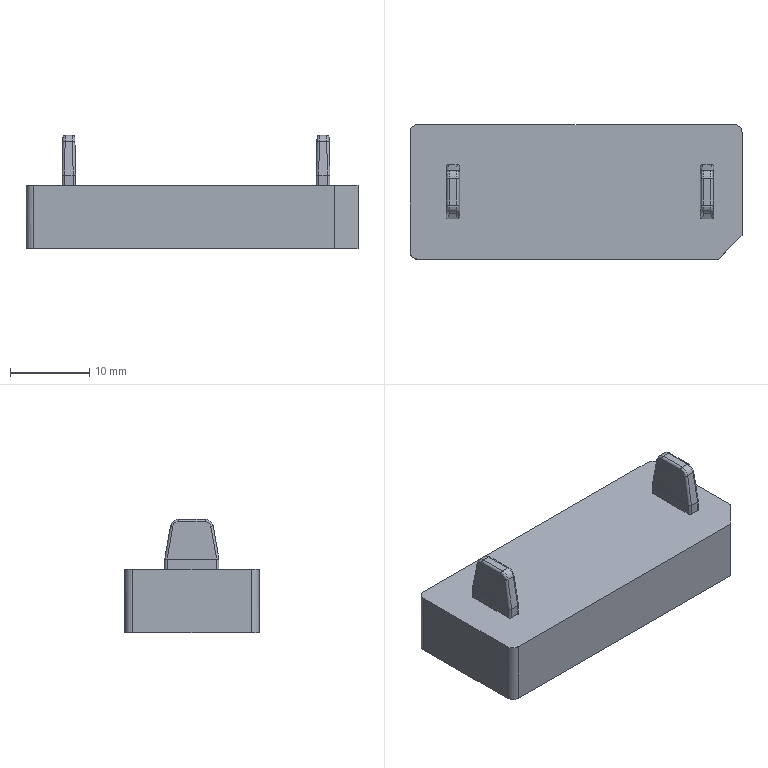NC program | PowerMill | posted by the shop | part box 42 x 17 x 14.346 mm
Lines 4335 to 5367 of 86217:
( TOOL ID   R1_1_1 )
( TOOL DIA. 2. TIP RAD 1. LENGTH 57.2 )
( Z = -2.198 )
T4 M6
T5
G91 G28 Z0
G0 G90 G54
M08
S18000 M3
X0 Y0 M8
G43 Z10.796 H4
X18.04 Y-3.123
Z-.918
G1 Z-2.118 F1200
X18.031 Y-3.133 Z-2.099 F2000
X18.016 Y-3.147 Z-2.074
X17.999 Y-3.164 Z-2.052
X17.932 Y-3.231 Z-2.005
X17.868 Y-3.296 Z-2.017
X17.813 Y-3.351 Z-2.056
X17.796 Y-3.368 Z-2.078
X17.67 Y-3.451 Z-2.068
X17.685 Y-3.436 Z-2.032
X17.706 Y-3.415 Z-1.992
X17.735 Y-3.386 Z-1.94
X17.754 Y-3.367 Z-1.908
X17.773 Y-3.348 Z-1.882
X17.792 Y-3.329 Z-1.86
X17.814 Y-3.307 Z-1.841
X17.837 Y-3.284 Z-1.825
X17.841 Y-3.28 Z-1.823
X17.905 Y-3.216 Z-1.806
X17.973 Y-3.148 Z-1.83
X18.035 Y-3.086 Z-1.898
X18.048 Y-3.073 Z-1.921
X18.061 Y-3.06 Z-1.949
X18.075 Y-3.045 Z-1.985
X18.092 Y-3.029 Z-2.033
X18.104 Y-3.016 Z-2.074
X18.113 Y-3.008 Z-2.106
X18.12 Y-3.001 Z-2.134
X18.122 Y-2.999 Z-2.142
X18.168 Y-2.91 Z-2.158
X18.165 Y-2.914 Z-2.137
X18.154 Y-2.924 Z-2.078
X18.143 Y-2.935 Z-2.023
X18.132 Y-2.947 Z-1.973
X18.12 Y-2.959 Z-1.928
X18.107 Y-2.972 Z-1.888
X18.093 Y-2.985 Z-1.851
X18.078 Y-3. Z-1.819
X18.062 Y-3.017 Z-1.79
X18.004 Y-3.075 Z-1.719
X17.937 Y-3.142 Z-1.681
X17.869 Y-3.21 Z-1.674
X17.858 Y-3.22 Z-1.677
X17.832 Y-3.246 Z-1.684
X17.807 Y-3.271 Z-1.695
X17.783 Y-3.296 Z-1.709
X17.76 Y-3.319 Z-1.726
X17.738 Y-3.341 Z-1.747
X17.716 Y-3.362 Z-1.771
X17.696 Y-3.383 Z-1.8
X17.675 Y-3.403 Z-1.834
X17.655 Y-3.423 Z-1.873
X17.634 Y-3.444 Z-1.921
X17.611 Y-3.468 Z-1.979
X17.581 Y-3.497 Z-2.059
X17.507 Y-3.529 Z-2.053
X17.52 Y-3.516 Z-2.012
X17.537 Y-3.499 Z-1.959
X17.559 Y-3.477 Z-1.893
X17.577 Y-3.459 Z-1.844
X17.594 Y-3.442 Z-1.805
X17.609 Y-3.427 Z-1.773
X17.623 Y-3.413 Z-1.75
X17.639 Y-3.397 Z-1.725
X17.661 Y-3.375 Z-1.696
X17.687 Y-3.349 Z-1.664
X17.712 Y-3.324 Z-1.638
X17.735 Y-3.301 Z-1.619
X17.756 Y-3.28 Z-1.605
X17.776 Y-3.26 Z-1.594
X17.796 Y-3.24 Z-1.585
X17.817 Y-3.219 Z-1.578
X17.84 Y-3.196 Z-1.571
X17.861 Y-3.175 Z-1.569
X17.882 Y-3.154
X17.902 Y-3.134 Z-1.57
X17.921 Y-3.115 Z-1.574
X17.944 Y-3.092 Z-1.583
X17.97 Y-3.066 Z-1.594
X18.034 Y-3.002 Z-1.644
X18.089 Y-2.947 Z-1.721
X18.106 Y-2.93 Z-1.756
X18.122 Y-2.914 Z-1.792
X18.136 Y-2.9 Z-1.83
X18.149 Y-2.887 Z-1.872
X18.16 Y-2.876 Z-1.918
X18.171 Y-2.865 Z-1.973
X18.18 Y-2.856 Z-2.031
X18.188 Y-2.848 Z-2.086
X18.195 Y-2.841 Z-2.138
X18.2 Y-2.836 Z-2.171
X18.223 Y-2.771 Z-2.183
X18.219 Y-2.775 Z-2.14
X18.212 Y-2.782 Z-2.072
X18.204 Y-2.79 Z-2.008
X18.196 Y-2.798 Z-1.949
X18.186 Y-2.807 Z-1.897
X18.175 Y-2.818 Z-1.846
X18.164 Y-2.83 Z-1.803
X18.149 Y-2.844 Z-1.756
X18.133 Y-2.86 Z-1.713
X18.116 Y-2.878 Z-1.675
X18.097 Y-2.896 Z-1.641
X18.077 Y-2.917 Z-1.609
X18.056 Y-2.937 Z-1.581
X18.033 Y-2.961 Z-1.556
X18.008 Y-2.986 Z-1.534
X17.982 Y-3.012 Z-1.515
X17.955 Y-3.038 Z-1.501
X17.928 Y-3.066 Z-1.49
X17.9 Y-3.093 Z-1.483
X17.872 Y-3.121 Z-1.48
X17.842 Y-3.151 Z-1.481
X17.813 Y-3.181 Z-1.486
X17.783 Y-3.211 Z-1.494
X17.753 Y-3.241 Z-1.507
X17.723 Y-3.27 Z-1.523
X17.694 Y-3.299 Z-1.544
X17.666 Y-3.328 Z-1.569
X17.638 Y-3.356 Z-1.597
X17.611 Y-3.382 Z-1.63
X17.587 Y-3.406 Z-1.663
X17.566 Y-3.428 Z-1.698
X17.545 Y-3.448 Z-1.736
X17.527 Y-3.467 Z-1.777
X17.509 Y-3.485 Z-1.822
X17.492 Y-3.502 Z-1.871
X17.475 Y-3.519 Z-1.926
X17.457 Y-3.536 Z-1.99
X17.441 Y-3.553 Z-2.047
X17.381 Y-3.57 Z-2.043
X17.399 Y-3.552 Z-1.974
X17.416 Y-3.535 Z-1.905
X17.431 Y-3.52 Z-1.851
X17.446 Y-3.505 Z-1.805
X17.462 Y-3.489 Z-1.762
X17.479 Y-3.472 Z-1.722
X17.497 Y-3.454 Z-1.684
X17.517 Y-3.434 Z-1.647
X17.539 Y-3.412 Z-1.611
X17.565 Y-3.386 Z-1.573
X17.593 Y-3.358 Z-1.539
X17.623 Y-3.328 Z-1.508
X17.653 Y-3.298 Z-1.481
X17.684 Y-3.267 Z-1.458
X17.716 Y-3.236 Z-1.439
X17.747 Y-3.204 Z-1.424
X17.779 Y-3.172 Z-1.413
X17.811 Y-3.141 Z-1.406
X17.842 Y-3.109 Z-1.403
X17.873 Y-3.078 Z-1.404
X17.903 Y-3.048 Z-1.408
X17.933 Y-3.018 Z-1.417
X17.961 Y-2.99 Z-1.429
X17.989 Y-2.962 Z-1.445
X18.016 Y-2.936 Z-1.465
X18.041 Y-2.91 Z-1.488
X18.065 Y-2.886 Z-1.515
X18.087 Y-2.864 Z-1.546
X18.109 Y-2.843 Z-1.58
X18.128 Y-2.823 Z-1.617
X18.146 Y-2.805 Z-1.657
X18.163 Y-2.788 Z-1.701
X18.177 Y-2.774 Z-1.748
X18.19 Y-2.761 Z-1.797
X18.199 Y-2.753 Z-1.836
X18.207 Y-2.744 Z-1.882
X18.215 Y-2.737 Z-1.928
X18.221 Y-2.73 Z-1.976
X18.227 Y-2.725 Z-2.034
X18.231 Y-2.72 Z-2.081
X18.235 Y-2.716 Z-2.129
X18.239 Y-2.712 Z-2.176
X18.241 Y-2.71 Z-2.193
X18.254 Y-2.655
X18.252 Y-2.656 Z-2.176
X18.247 Y-2.662 Z-2.096
X18.24 Y-2.669 Z-2.012
X18.232 Y-2.676 Z-1.934
X18.223 Y-2.685 Z-1.865
X18.213 Y-2.696 Z-1.802
X18.2 Y-2.709 Z-1.743
X18.188 Y-2.721 Z-1.697
X18.172 Y-2.736 Z-1.648
X18.155 Y-2.754 Z-1.602
X18.136 Y-2.773 Z-1.56
X18.115 Y-2.793 Z-1.522
X18.093 Y-2.815 Z-1.487
X18.07 Y-2.839 Z-1.456
X18.045 Y-2.863 Z-1.428
X18.019 Y-2.889 Z-1.404
X17.992 Y-2.917 Z-1.383
X17.964 Y-2.945 Z-1.366
X17.934 Y-2.975 Z-1.352
X17.904 Y-3.005 Z-1.342
X17.873 Y-3.036 Z-1.336
X17.841 Y-3.068 Z-1.333
X17.808 Y-3.1 Z-1.335
X17.775 Y-3.133 Z-1.34
X17.742 Y-3.166 Z-1.349
X17.709 Y-3.2 Z-1.363
X17.676 Y-3.233 Z-1.38
X17.643 Y-3.266 Z-1.402
X17.611 Y-3.298 Z-1.427
X17.58 Y-3.329 Z-1.456
X17.55 Y-3.359 Z-1.489
X17.526 Y-3.383 Z-1.519
X17.5 Y-3.408 Z-1.555
X17.477 Y-3.432 Z-1.592
X17.454 Y-3.454 Z-1.631
X17.434 Y-3.475 Z-1.673
X17.415 Y-3.494 Z-1.717
X17.398 Y-3.511 Z-1.763
X17.382 Y-3.527 Z-1.813
X17.366 Y-3.542 Z-1.866
X17.352 Y-3.557 Z-1.924
X17.338 Y-3.571 Z-1.985
X17.325 Y-3.584 Z-2.039
X17.272 Y-3.594 Z-2.036
X17.286 Y-3.581 Z-1.974
X17.301 Y-3.566 Z-1.907
X17.318 Y-3.549 Z-1.837
X17.334 Y-3.532 Z-1.778
X17.351 Y-3.515 Z-1.728
X17.368 Y-3.498 Z-1.682
X17.387 Y-3.479 Z-1.639
X17.407 Y-3.459 Z-1.599
X17.428 Y-3.438 Z-1.56
X17.452 Y-3.415 Z-1.521
X17.48 Y-3.386 Z-1.48
X17.51 Y-3.356 Z-1.441
X17.542 Y-3.324 Z-1.406
X17.575 Y-3.292 Z-1.375
X17.608 Y-3.258 Z-1.348
X17.642 Y-3.224 Z-1.325
X17.677 Y-3.19 Z-1.306
X17.711 Y-3.155 Z-1.291
X17.745 Y-3.121 Z-1.28
X17.78 Y-3.087 Z-1.273
X17.813 Y-3.053 Z-1.27
X17.847 Y-3.02 Z-1.271
X17.88 Y-2.987 Z-1.276
X17.91 Y-2.956 Z-1.284
X17.941 Y-2.925 Z-1.296
X17.972 Y-2.895 Z-1.311
X18. Y-2.866 Z-1.33
X18.028 Y-2.838 Z-1.352
X18.054 Y-2.812 Z-1.378
X18.079 Y-2.787 Z-1.407
X18.103 Y-2.763 Z-1.44
X18.125 Y-2.741 Z-1.476
X18.146 Y-2.721 Z-1.515
X18.164 Y-2.702 Z-1.559
X18.182 Y-2.685 Z-1.605
X18.197 Y-2.669 Z-1.655
X18.211 Y-2.656 Z-1.709
X18.222 Y-2.644 Z-1.764
X18.231 Y-2.635 Z-1.816
X18.239 Y-2.628 Z-1.87
X18.245 Y-2.621 Z-1.923
X18.25 Y-2.616 Z-1.985
X18.254 Y-2.612 Z-2.039
X18.257 Y-2.609 Z-2.093
X18.26 Y-2.606 Z-2.148
X18.262 Y-2.605 Z-2.173
X18.268 Y-2.556 Z-2.147
X18.267 Y-2.557 Z-2.131
X18.262 Y-2.562 Z-2.033
X18.256 Y-2.567 Z-1.94
X18.25 Y-2.574 Z-1.865
X18.241 Y-2.583 Z-1.798
X18.231 Y-2.593 Z-1.733
X18.219 Y-2.605 Z-1.675
X18.206 Y-2.618 Z-1.62
X18.19 Y-2.634 Z-1.568
X18.173 Y-2.651 Z-1.52
X18.154 Y-2.67 Z-1.475
X18.134 Y-2.69 Z-1.436
X18.112 Y-2.712 Z-1.399
X18.088 Y-2.736 Z-1.365
X18.062 Y-2.761 Z-1.334
X18.035 Y-2.789 Z-1.306
X18.007 Y-2.817 Z-1.282
X17.977 Y-2.847 Z-1.261
X17.946 Y-2.878 Z-1.244
X17.914 Y-2.91 Z-1.23
X17.881 Y-2.943 Z-1.22
X17.848 Y-2.976 Z-1.214
X17.814 Y-3.01 Z-1.212
X17.779 Y-3.044 Z-1.213
X17.745 Y-3.079 Z-1.218
X17.709 Y-3.115 Z-1.228
X17.673 Y-3.151 Z-1.241
X17.638 Y-3.186 Z-1.258
X17.602 Y-3.222 Z-1.279
X17.567 Y-3.256 Z-1.305
X17.533 Y-3.291 Z-1.334
X17.499 Y-3.325 Z-1.368
X17.468 Y-3.356 Z-1.403
X17.438 Y-3.386 Z-1.442
X17.409 Y-3.415 Z-1.484
X17.382 Y-3.442 Z-1.531
X17.355 Y-3.469 Z-1.581
X17.335 Y-3.489 Z-1.625
X17.317 Y-3.507 Z-1.668
X17.301 Y-3.523 Z-1.712
X17.286 Y-3.538 Z-1.756
X17.273 Y-3.551 Z-1.802
X17.262 Y-3.562 Z-1.848
X17.251 Y-3.573 Z-1.896
X17.241 Y-3.583 Z-1.944
X17.231 Y-3.593 Z-1.992
X17.222 Y-3.602 Z-2.034
X17.174 Y-3.608 Z-2.033
X17.195 Y-3.586 Z-1.923
X17.212 Y-3.569 Z-1.845
X17.228 Y-3.553 Z-1.78
X17.245 Y-3.536 Z-1.722
X17.263 Y-3.519 Z-1.67
X17.282 Y-3.5 Z-1.62
X17.302 Y-3.479 Z-1.574
X17.324 Y-3.457 Z-1.529
X17.348 Y-3.433 Z-1.485
X17.374 Y-3.408 Z-1.443
X17.403 Y-3.378 Z-1.399
X17.435 Y-3.347 Z-1.358
X17.468 Y-3.313 Z-1.321
X17.503 Y-3.279 Z-1.287
X17.538 Y-3.243 Z-1.257
X17.575 Y-3.207 Z-1.23
X17.611 Y-3.17 Z-1.208
X17.648 Y-3.133 Z-1.19
X17.685 Y-3.096 Z-1.176
X17.722 Y-3.059 Z-1.166
X17.759 Y-3.023 Z-1.16
X17.795 Y-2.986 Z-1.158
X17.831 Y-2.951 Z-1.16
X17.866 Y-2.916 Z-1.166
X17.9 Y-2.882 Z-1.175
X17.933 Y-2.848 Z-1.188
X17.965 Y-2.816 Z-1.205
X17.996 Y-2.786 Z-1.225
X18.025 Y-2.756 Z-1.248
X18.054 Y-2.728 Z-1.276
X18.08 Y-2.701 Z-1.306
X18.105 Y-2.676 Z-1.34
X18.129 Y-2.652 Z-1.378
X18.151 Y-2.631 Z-1.418
X18.171 Y-2.611 Z-1.462
X18.189 Y-2.592 Z-1.508
X18.205 Y-2.576 Z-1.558
X18.219 Y-2.562 Z-1.61
X18.231 Y-2.55 Z-1.665
X18.241 Y-2.54 Z-1.725
X18.251 Y-2.531 Z-1.792
X18.259 Y-2.523 Z-1.871
X18.265 Y-2.516 Z-1.962
X18.269 Y-2.512 Z-2.045
X18.272 Y-2.509 Z-2.114
X18.273 Z-2.122
X18.275 Y-2.464 Z-2.099
Z-2.085
X18.272 Y-2.467 Z-1.99
X18.266 Y-2.473 Z-1.891
X18.26 Y-2.479 Z-1.808
X18.252 Y-2.487 Z-1.736
X18.243 Y-2.496 Z-1.672
X18.233 Y-2.506 Z-1.615
X18.22 Y-2.519 Z-1.562
X18.206 Y-2.533 Z-1.511
X18.19 Y-2.549 Z-1.462
X18.172 Y-2.567 Z-1.417
X18.152 Y-2.587 Z-1.374
X18.13 Y-2.609 Z-1.334
X18.107 Y-2.632 Z-1.297
X18.082 Y-2.658 Z-1.263
X18.055 Y-2.684 Z-1.232
X18.026 Y-2.713 Z-1.204
X17.996 Y-2.743 Z-1.18
X17.964 Y-2.775 Z-1.159
X17.931 Y-2.808 Z-1.142
X17.897 Y-2.842 Z-1.128
X17.861 Y-2.878 Z-1.117
X17.825 Y-2.914 Z-1.111
X17.788 Y-2.951 Z-1.108
X17.751 Y-2.988 Z-1.109
X17.714 Y-3.025 Z-1.114
X17.676 Y-3.063 Z-1.124
X17.638 Y-3.101 Z-1.137
X17.6 Y-3.139 Z-1.154
X17.562 Y-3.177 Z-1.176
X17.525 Y-3.215 Z-1.201
X17.488 Y-3.251 Z-1.231
X17.452 Y-3.287 Z-1.264
X17.417 Y-3.322 Z-1.301
X17.383 Y-3.356 Z-1.342
X17.351 Y-3.388 Z-1.385
X17.321 Y-3.418 Z-1.432
X17.293 Y-3.446 Z-1.482
X17.267 Y-3.472 Z-1.536
X17.242 Y-3.497 Z-1.592
X17.225 Y-3.514 Z-1.635
X17.21 Y-3.529 Z-1.678
X17.195 Y-3.544 Z-1.723
X17.182 Y-3.557 Z-1.768
X17.171 Y-3.568 Z-1.815
X17.157 Y-3.582 Z-1.877
X17.146 Y-3.593 Z-1.935
X17.137 Y-3.602 Z-1.984
X17.128 Y-3.611 Z-2.032
X17.084 Y-3.613 Z-2.03
X17.104 Y-3.593 Z-1.919
X17.119 Y-3.577 Z-1.841
X17.134 Y-3.563 Z-1.776
X17.149 Y-3.548 Z-1.719
X17.165 Y-3.531 Z-1.666
X17.183 Y-3.514 Z-1.616
X17.202 Y-3.495 Z-1.568
X17.222 Y-3.474 Z-1.521
X17.244 Y-3.452 Z-1.475
X17.268 Y-3.428 Z-1.431
X17.294 Y-3.402 Z-1.386
X17.326 Y-3.371 Z-1.339
X17.358 Y-3.338 Z-1.295
X17.393 Y-3.304 Z-1.254
X17.429 Y-3.268 Z-1.217
X17.465 Y-3.231 Z-1.184
X17.503 Y-3.194 Z-1.155
X17.541 Y-3.155 Z-1.129
X17.58 Y-3.117 Z-1.108
X17.619 Y-3.078 Z-1.091
X17.658 Y-3.039 Z-1.078
X17.697 Y-3. Z-1.068
X17.736 Y-2.961 Z-1.063
X17.775 Y-2.921 Z-1.061
X17.813 Y-2.884 Z-1.064
X17.849 Y-2.847 Z-1.07
X17.885 Y-2.811 Z-1.08
X17.921 Y-2.776 Z-1.094
X17.955 Y-2.742 Z-1.111
X17.987 Y-2.709 Z-1.132
X18.019 Y-2.678 Z-1.157
X18.048 Y-2.648 Z-1.185
X18.077 Y-2.62 Z-1.216
X18.103 Y-2.594 Z-1.25
X18.128 Y-2.569 Z-1.288
X18.15 Y-2.546 Z-1.328
X18.171 Y-2.526 Z-1.37
X18.189 Y-2.507 Z-1.416
X18.206 Y-2.491 Z-1.463
X18.221 Y-2.476 Z-1.516
X18.234 Y-2.463 Z-1.572
X18.245 Y-2.451 Z-1.633
X18.255 Y-2.442 Z-1.7
X18.263 Y-2.434 Z-1.773
X18.269 Y-2.428 Z-1.856
X18.273 Y-2.423 Z-1.952
X18.277 Y-2.42 Z-2.071
Y-2.377 Z-2.041
X18.276 Y-2.379 Z-1.978
X18.273 Y-2.382 Z-1.875
X18.268 Y-2.386 Z-1.788
X18.262 Y-2.392 Z-1.712
X18.254 Y-2.4 Z-1.644
X18.244 Y-2.41 Z-1.581
X18.233 Y-2.422 Z-1.522
X18.219 Y-2.436 Z-1.466
X18.203 Y-2.451 Z-1.416
X18.186 Y-2.468 Z-1.368
X18.166 Y-2.488 Z-1.322
X18.145 Y-2.509 Z-1.279
X18.121 Y-2.533 Z-1.24
X18.096 Y-2.558 Z-1.203
X18.069 Y-2.586 Z-1.169
X18.04 Y-2.614 Z-1.138
X18.009 Y-2.645 Z-1.111
X17.977 Y-2.677 Z-1.087
X17.944 Y-2.71 Z-1.067
X17.91 Y-2.745 Z-1.05
X17.874 Y-2.78 Z-1.036
X17.837 Y-2.817 Z-1.026
X17.799 Y-2.856 Z-1.02
X17.76 Y-2.894 Z-1.017
X17.72 Y-2.934 Z-1.019
X17.681 Y-2.973 Z-1.024
X17.641 Y-3.013 Z-1.033
X17.601 Y-3.053 Z-1.047
X17.561 Y-3.093 Z-1.064
X17.521 Y-3.133 Z-1.086
X17.482 Y-3.172 Z-1.111
X17.443 Y-3.211 Z-1.141
X17.406 Y-3.248 Z-1.174
X17.371 Y-3.284 Z-1.21
X17.335 Y-3.319 Z-1.25
X17.301 Y-3.354 Z-1.294
X17.268 Y-3.386 Z-1.342
X17.237 Y-3.417 Z-1.392
X17.209 Y-3.446 Z-1.446
X17.182 Y-3.472 Z-1.502
X17.162 Y-3.492 Z-1.548
X17.143 Y-3.511 Z-1.596
X17.126 Y-3.528 Z-1.645
X17.111 Y-3.543 Z-1.694
X17.097 Y-3.557 Z-1.745
X17.084 Y-3.571 Z-1.801
X17.07 Y-3.584 Z-1.865
X17.055 Y-3.599 Z-1.95
X17.041 Y-3.613 Z-2.028
X16.999 Z-2.027
X17.009 Y-3.603 Z-1.97
X17.02 Y-3.592 Z-1.91
X17.032 Y-3.58 Z-1.843
X17.047 Y-3.564 Z-1.77
X17.062 Y-3.549 Z-1.71
X17.078 Y-3.534 Z-1.657
X17.094 Y-3.518 Z-1.608
X17.111 Y-3.501 Z-1.56
X17.13 Y-3.482 Z-1.513
X17.15 Y-3.461 Z-1.467
X17.178 Y-3.433 Z-1.41
X17.208 Y-3.403 Z-1.356
X17.24 Y-3.372 Z-1.304
X17.273 Y-3.338 Z-1.257
X17.308 Y-3.304 Z-1.212
X17.344 Y-3.267 Z-1.172
X17.382 Y-3.23 Z-1.134
X17.42 Y-3.191 Z-1.101
X17.46 Y-3.152 Z-1.071
X17.5 Y-3.112 Z-1.045
X17.54 Y-3.071 Z-1.024
X17.581 Y-3.031 Z-1.006
X17.622 Y-2.99 Z-.992
X17.663 Y-2.949 Z-.982
X17.704 Y-2.908 Z-.977
X17.744 Y-2.868 Z-.975
X17.784 Y-2.828 Z-.978
X17.823 Y-2.789 Z-.984
X17.861 Y-2.75 Z-.994
X17.899 Y-2.713 Z-1.007
X17.934 Y-2.677 Z-1.025
X17.969 Y-2.643 Z-1.045
X18.001 Y-2.61 Z-1.069
X18.033 Y-2.579 Z-1.097
X18.062 Y-2.55 Z-1.127
X18.089 Y-2.522 Z-1.16
X18.115 Y-2.497 Z-1.195
X18.139 Y-2.473 Z-1.234
X18.161 Y-2.451 Z-1.275
X18.181 Y-2.431 Z-1.318
X18.199 Y-2.413 Z-1.364
X18.215 Y-2.397 Z-1.413
X18.229 Y-2.383 Z-1.466
X18.241 Y-2.371 Z-1.522
X18.252 Y-2.36 Z-1.582
X18.26 Y-2.352 Z-1.648
X18.267 Y-2.345 Z-1.72
X18.271 Y-2.34 Z-1.802
X18.275 Y-2.337 Z-1.899
X18.277 Y-2.335 Z-2.012
X18.276 Y-2.293 Z-1.984
X18.275 Y-2.295 Z-1.88
X18.272 Y-2.297 Z-1.779
X18.268 Y-2.302 Z-1.697
X18.262 Y-2.308 Z-1.625
X18.254 Y-2.315 Z-1.56
X18.244 Y-2.325 Z-1.501
X18.232 Y-2.337 Z-1.445
X18.218 Y-2.351 Z-1.391
X18.202 Y-2.367 Z-1.34
X18.183 Y-2.386 Z-1.292
X18.163 Y-2.406 Z-1.248
X18.141 Y-2.428 Z-1.205
X18.116 Y-2.453 Z-1.166
X18.09 Y-2.48 Z-1.128
X18.061 Y-2.508 Z-1.094
X18.031 Y-2.539 Z-1.062
X17.998 Y-2.571 Z-1.034
X17.965 Y-2.605 Z-1.009
X17.929 Y-2.64 Z-.988
X17.893 Y-2.676 Z-.97
X17.855 Y-2.714 Z-.956
X17.817 Y-2.753 Z-.945
X17.777 Y-2.792 Z-.939
X17.737 Y-2.833 Z-.936
X17.696 Y-2.874 Z-.937
X17.654 Y-2.915 Z-.942
X17.613 Y-2.957 Z-.951
X17.571 Y-2.999 Z-.964
X17.529 Y-3.04 Z-.981
X17.488 Y-3.082 Z-1.002
X17.447 Y-3.123 Z-1.027
X17.406 Y-3.163 Z-1.056
X17.367 Y-3.202 Z-1.089
X17.329 Y-3.241 Z-1.126
X17.291 Y-3.278 Z-1.166
X17.255 Y-3.314 Z-1.21
X17.221 Y-3.349 Z-1.257
X17.188 Y-3.382 Z-1.308
X17.156 Y-3.413 Z-1.362
X17.127 Y-3.442 Z-1.419
X17.099 Y-3.47 Z-1.479
X17.079 Y-3.491 Z-1.53
X17.059 Y-3.51 Z-1.581
X17.042 Y-3.528 Z-1.634
X17.025 Y-3.544 Z-1.689
X17.009 Y-3.56 Z-1.752
X16.993 Y-3.576 Z-1.826
X16.979 Y-3.59 Z-1.898
X16.968 Y-3.602 Z-1.964
X16.957 Y-3.612 Z-2.025
X16.915 Z-2.023
X16.925 Y-3.602 Z-1.964
X16.936 Y-3.591 Z-1.904
X16.949 Y-3.578 Z-1.836
X16.965 Y-3.562 Z-1.762
X16.98 Y-3.547 Z-1.702
X16.996 Y-3.531 Z-1.646
X17.013 Y-3.514 Z-1.591
X17.033 Y-3.494 Z-1.537
X17.053 Y-3.474 Z-1.484
X17.075 Y-3.452 Z-1.432
X17.102 Y-3.425 Z-1.377
X17.132 Y-3.395 Z-1.321
X17.165 Y-3.362 Z-1.267
X17.2 Y-3.327 Z-1.215
X17.236 Y-3.291 Z-1.167
X17.272 Y-3.254 Z-1.124
X17.309 Y-3.218 Z-1.086
X17.346 Y-3.181 Z-1.052
X17.386 Y-3.141 Z-1.019
X17.428 Y-3.099 Z-.99
X17.469 Y-3.057 Z-.965
X17.512 Y-3.015 Z-.944
X17.554 Y-2.973 Z-.927
X17.596 Y-2.931 Z-.914
X17.639 Y-2.888 Z-.905
X17.681 Y-2.846 Z-.9
X17.722 Y-2.805 Z-.899
X17.761 Y-2.766 Z-.901
X17.801 Y-2.725 Z-.908
X17.841 Y-2.686 Z-.918
X17.88 Y-2.647 Z-.932
X17.918 Y-2.609 Z-.95
X17.954 Y-2.573 Z-.971
X17.988 Y-2.539 Z-.995
X18.021 Y-2.506 Z-1.023
X18.052 Y-2.475 Z-1.054
X18.081 Y-2.446 Z-1.088
X18.109 Y-2.418 Z-1.124
X18.134 Y-2.393 Z-1.163
X18.157 Y-2.37 Z-1.205
X18.178 Y-2.349 Z-1.249
X18.197 Y-2.33 Z-1.295
X18.213 Y-2.314 Z-1.344
X18.228 Y-2.299 Z-1.395
X18.24 Y-2.287 Z-1.447
X18.25 Y-2.277 Z-1.502
X18.259 Y-2.268 Z-1.564
X18.265 Y-2.262 Z-1.632
X18.27 Y-2.257 Z-1.708
X18.273 Y-2.254 Z-1.797
X18.275 Y-2.252 Z-1.913
Y-2.251 Z-1.951
Y-2.21 Z-1.903
X18.274 Y-2.211 Z-1.819
X18.272 Y-2.213 Z-1.719
X18.268 Y-2.217 Z-1.638
X18.262 Y-2.222 Z-1.568
X18.255 Y-2.229 Z-1.504
X18.246 Y-2.239 Z-1.446
X18.234 Y-2.25 Z-1.392
X18.221 Y-2.264 Z-1.34
X18.205 Y-2.28 Z-1.289
X18.186 Y-2.298 Z-1.241
X18.166 Y-2.319 Z-1.195
X18.143 Y-2.342 Z-1.152
X18.118 Y-2.367 Z-1.111
X18.091 Y-2.394 Z-1.072
X18.062 Y-2.423 Z-1.037
X18.031 Y-2.454 Z-1.004
X17.998 Y-2.487 Z-.975
X17.963 Y-2.521 Z-.948
X17.927 Y-2.557 Z-.925
X17.89 Y-2.595 Z-.906
X17.851 Y-2.633 Z-.89
X17.811 Y-2.673 Z-.877
X17.771 Y-2.714 Z-.869
X17.728 Y-2.756 Z-.864
X17.686 Y-2.799 Z-.863
X17.643 Y-2.841 Z-.866
X17.6 Y-2.884 Z-.873
X17.557 Y-2.927 Z-.884
X17.514 Y-2.97 Z-.899
X17.471 Y-3.013 Z-.919
X17.429 Y-3.055 Z-.942
X17.387 Y-3.097 Z-.969
X17.346 Y-3.138 Z-1.
X17.306 Y-3.178 Z-1.034
X17.266 Y-3.218 Z-1.073
X17.228 Y-3.257 Z-1.115
X17.191 Y-3.294 Z-1.16
X17.156 Y-3.329 Z-1.208
X17.122 Y-3.362 Z-1.259
X17.091 Y-3.394 Z-1.313
X17.061 Y-3.424 Z-1.371
X17.032 Y-3.452 Z-1.432
X17.005 Y-3.479 Z-1.497
X16.98 Y-3.505 Z-1.565
X16.962 Y-3.522 Z-1.617
X16.946 Y-3.539 Z-1.67
X16.931 Y-3.553 Z-1.724
X16.918 Y-3.566 Z-1.779
X16.903 Y-3.581 Z-1.85
X16.893 Y-3.592 Z-1.908
X16.883 Y-3.602 Z-1.965
X16.873 Y-3.612 Z-2.021
X16.831 Y-3.611 Z-2.018
X16.842 Y-3.6 Z-1.955
X16.853 Y-3.589 Z-1.891
X16.866 Y-3.577 Z-1.828
X16.88 Y-3.562 Z-1.763
X16.897 Y-3.545 Z-1.695
X16.917 Y-3.526 Z-1.627
X16.937 Y-3.505 Z-1.565
X16.959 Y-3.483 Z-1.508
X16.982 Y-3.46 Z-1.451
X17.007 Y-3.435 Z-1.396
X17.033 Y-3.409 Z-1.342
X17.059 Y-3.384 Z-1.292
X17.087 Y-3.355 Z-1.242
X17.119 Y-3.323 Z-1.193
X17.155 Y-3.287 Z-1.143
X17.193 Y-3.249 Z-1.095
X17.233 Y-3.209 Z-1.051
X17.274 Y-3.168 Z-1.01
X17.315 Y-3.128 Z-.975
X17.354 Y-3.088 Z-.944
X17.394 Y-3.048 Z-.917
X17.433 Y-3.009 Z-.895
X17.477 Y-2.965 Z-.874
X17.521 Y-2.921 Z-.857
X17.565 Y-2.877 Z-.844
X17.609 Y-2.833 Z-.835
X17.653 Y-2.789 Z-.83
X17.696 Y-2.746 Z-.829
X17.739 Y-2.704 Z-.832
X17.78 Y-2.662 Z-.839
X17.821 Y-2.621 Z-.85
X17.861 Y-2.581 Z-.864
X17.9 Y-2.542 Z-.882
X17.938 Y-2.505 Z-.904
X17.974 Y-2.469 Z-.929
X18.008 Y-2.434 Z-.957
X18.04 Y-2.402 Z-.988
X18.071 Y-2.371 Z-1.022
X18.1 Y-2.342 Z-1.059
X18.126 Y-2.316 Z-1.099
X18.151 Y-2.291 Z-1.141
X18.173 Y-2.269 Z-1.186
X18.193 Y-2.249 Z-1.233
X18.211 Y-2.231 Z-1.282
X18.226 Y-2.216 Z-1.333
X18.239 Y-2.203 Z-1.385
X18.249 Y-2.193 Z-1.439
X18.258 Y-2.184 Z-1.497
X18.264 Y-2.178 Z-1.561
X18.269 Y-2.173 Z-1.632
X18.272 Y-2.17 Z-1.716
X18.273 Y-2.169 Z-1.826
X18.274 Y-2.168 Z-1.854
X18.273 Y-2.127 Z-1.805
X18.272 Y-2.128 Z-1.712
X18.269 Y-2.13 Z-1.623
X18.265 Y-2.134 Z-1.55
X18.259 Y-2.14 Z-1.485
X18.252 Y-2.148 Z-1.427
X18.242 Y-2.158 Z-1.373
X18.23 Y-2.17 Z-1.323
X18.215 Y-2.185 Z-1.271
X18.197 Y-2.202 Z-1.221
X18.177 Y-2.223 Z-1.173
X18.155 Y-2.245 Z-1.126
X18.13 Y-2.27 Z-1.083
X18.103 Y-2.296 Z-1.042
X18.074 Y-2.325 Z-1.003
X18.044 Y-2.356 Z-.968
X18.011 Y-2.389 Z-.936
X17.977 Y-2.423 Z-.906
X17.941 Y-2.459 Z-.88
X17.903 Y-2.496 Z-.858
X17.864 Y-2.535 Z-.839
X17.824 Y-2.575 Z-.823
X17.783 Y-2.616 Z-.811
X17.741 Y-2.659 Z-.802
X17.698 Y-2.702 Z-.798
X17.654 Y-2.745 Z-.797
X17.61 Y-2.789 Z-.8
X17.566 Y-2.834 Z-.808
X17.522 Y-2.878 Z-.819
X17.477 Y-2.922 Z-.834
X17.433 Y-2.967 Z-.854
X17.389 Y-3.01 Z-.877
X17.346 Y-3.054 Z-.904
X17.303 Y-3.096 Z-.936
X17.26 Y-3.139 Z-.972
X17.218 Y-3.182 Z-1.012
X17.176 Y-3.224 Z-1.056
X17.142 Y-3.258 Z-1.097
X17.107 Y-3.292 Z-1.143
X17.073 Y-3.327 Z-1.194
X17.039 Y-3.361 Z-1.251
X17.005 Y-3.394 Z-1.312
X16.973 Y-3.427 Z-1.378
X16.949 Y-3.45 Z-1.43
X16.927 Y-3.473 Z-1.482
X16.906 Y-3.494 Z-1.536
X16.886 Y-3.514 Z-1.591
X16.868 Y-3.532 Z-1.647
X16.851 Y-3.549 Z-1.707
X16.834 Y-3.565 Z-1.775
X16.821 Y-3.578 Z-1.836
X16.81 Y-3.59 Z-1.896
X16.799 Y-3.601 Z-1.956
X16.789 Y-3.611 Z-2.016
X16.747 Y-3.61 Z-2.013
X16.757 Y-3.6 Z-1.954
X16.768 Y-3.589 Z-1.895
X16.779 Y-3.578 Z-1.836
X16.792 Y-3.565 Z-1.775
X16.808 Y-3.549 Z-1.708
X16.825 Y-3.532 Z-1.648
X16.843 Y-3.514 Z-1.593
X16.862 Y-3.495 Z-1.539
X16.883 Y-3.474 Z-1.485
X16.905 Y-3.452 Z-1.433
X16.928 Y-3.429 Z-1.381
X16.961 Y-3.396 Z-1.314
X16.996 Y-3.361 Z-1.25
X17.033 Y-3.324 Z-1.189
X17.072 Y-3.286 Z-1.131
X17.108 Y-3.249 Z-1.081
X17.146 Y-3.211 Z-1.035
X17.186 Y-3.172 Z-.992
X17.227 Y-3.13 Z-.952
X17.27 Y-3.087 Z-.916
X17.315 Y-3.042 Z-.882
X17.361 Y-2.996 Z-.853
X17.408 Y-2.949 Z-.827
X17.451 Y-2.907 Z-.807
X17.494 Y-2.863 Z-.791
X17.539 Y-2.819 Z-.779
X17.583 Y-2.774 Z-.771
X17.628 Y-2.729 Z-.767
X17.673 Y-2.684 Z-.766
X17.717 Y-2.64 Z-.77
X17.761 Y-2.596 Z-.778
X17.805 Y-2.552 Z-.79
X17.845 Y-2.512 Z-.804
X17.885 Y-2.473 Z-.823
X17.923 Y-2.434 Z-.845
X17.96 Y-2.397 Z-.87
X17.996 Y-2.362 Z-.899
X18.03 Y-2.328 Z-.931
X18.062 Y-2.296 Z-.967
X18.092 Y-2.265 Z-1.005
X18.12 Y-2.237 Z-1.046
X18.146 Y-2.212 Z-1.089
X18.169 Y-2.188 Z-1.134
X18.19 Y-2.167 Z-1.182
X18.209 Y-2.148 Z-1.231
X18.224 Y-2.133 Z-1.279
X18.237 Y-2.121 Z-1.328
X18.247 Y-2.11 Z-1.38
X18.256 Y-2.101 Z-1.437
X18.263 Y-2.094 Z-1.499
X18.268 Y-2.09 Z-1.568
X18.271 Y-2.087 Z-1.649
X18.272 Y-2.085 Z-1.751
Z-1.756
X18.271 Y-2.043 Z-1.721
Z-1.708
Y-2.044 Z-1.649
X18.269 Y-2.045 Z-1.586
X18.266 Y-2.048 Z-1.519
X18.261 Y-2.053 Z-1.459
X18.255 Y-2.06 Z-1.407
X18.246 Y-2.068 Z-1.358
X18.236 Y-2.078 Z-1.312
X18.225 Y-2.09 Z-1.267
X18.211 Y-2.103 Z-1.223
X18.196 Y-2.119 Z-1.179
X18.177 Y-2.138 Z-1.132
X18.155 Y-2.16 Z-1.086
X18.131 Y-2.184 Z-1.043
X18.104 Y-2.21 Z-1.002
X18.076 Y-2.239 Z-.962
X18.044 Y-2.27 Z-.926
X18.011 Y-2.304 Z-.892
X17.976 Y-2.339 Z-.861
X17.939 Y-2.376 Z-.833
X17.9 Y-2.415 Z-.809
X17.86 Y-2.455 Z-.787
X17.819 Y-2.496 Z-.77
X17.776 Y-2.539 Z-.756
X17.733 Y-2.582 Z-.746
X17.689 Y-2.626 Z-.739
X17.644 Y-2.671 Z-.737
X17.599 Y-2.716 Z-.739
X17.553 Y-2.761 Z-.744
X17.508 Y-2.807 Z-.754
X17.463 Y-2.852 Z-.767
X17.418 Y-2.897 Z-.785
X17.373 Y-2.942 Z-.806
X17.329 Y-2.986 Z-.832
X17.289 Y-3.026 Z-.859
X17.25 Y-3.065 Z-.887
X17.212 Y-3.103 Z-.918
X17.174 Y-3.141 Z-.953
X17.137 Y-3.178 Z-.991
X17.099 Y-3.215 Z-1.034
X17.063 Y-3.252 Z-1.081
X17.029 Y-3.286 Z-1.13
X16.996 Y-3.318 Z-1.18
X16.965 Y-3.349 Z-1.231
X16.935 Y-3.38 Z-1.284
X16.901 Y-3.414 Z-1.35
X16.869 Y-3.446 Z-1.418
X16.839 Y-3.476 Z-1.489
X16.812 Y-3.503 Z-1.561
X16.787 Y-3.528 Z-1.636
X16.77 Y-3.545 Z-1.693
X16.755 Y-3.56 Z-1.751
X16.742 Y-3.573 Z-1.81
X16.726 Y-3.588 Z-1.889
X16.715 Y-3.6 Z-1.952
X16.705 Y-3.61 Z-2.012
X16.662
X16.673 Y-3.6 Z-1.951
X16.683 Y-3.589 Z-1.891
X16.695 Y-3.577 Z-1.831
X16.708 Y-3.565 Z-1.772
X16.724 Y-3.548 Z-1.705
X16.74 Y-3.532 Z-1.648
X16.758 Y-3.514 Z-1.592
X16.778 Y-3.494 Z-1.537
X16.8 Y-3.473 Z-1.483
X16.822 Y-3.45 Z-1.43
X16.845 Y-3.427 Z-1.378
X16.877 Y-3.395 Z-1.314
X16.913 Y-3.36 Z-1.249
X16.953 Y-3.319 Z-1.18
X16.992 Y-3.281 Z-1.121
X17.027 Y-3.245 Z-1.07
X17.065 Y-3.207 Z-1.021
X17.105 Y-3.167 Z-.975
X17.148 Y-3.125 Z-.931
X17.192 Y-3.081 Z-.891
X17.237 Y-3.036 Z-.854
X17.282 Y-2.99 Z-.822
X17.327 Y-2.945 Z-.793
X17.373 Y-2.9 Z-.769
X17.417 Y-2.855 Z-.75
X17.461 Y-2.811 Z-.735
X17.507 Y-2.765 Z-.722
X17.554 Y-2.719 Z-.714
X17.6 Y-2.673 Z-.71
X17.645 Y-2.627
X17.69 Y-2.582 Z-.713
X17.735 Y-2.538 Z-.721
X17.778 Y-2.494 Z-.732
X17.821 Y-2.452 Z-.747
X17.862 Y-2.41 Z-.766
X17.903 Y-2.37 Z-.789
X17.941 Y-2.331 Z-.814
X17.978 Y-2.294 Z-.843
X18.013 Y-2.259 Z-.875
X18.046 Y-2.226 Z-.91
X18.078 Y-2.195 Z-.948
X18.107 Y-2.166 Z-.989
X18.134 Y-2.139 Z-1.032
X18.158 Y-2.114 Z-1.077
X18.181 Y-2.091 Z-1.125
X18.201 Y-2.071 Z-1.175
X18.219 Y-2.054 Z-1.227
X18.232 Y-2.04 Z-1.275
X18.244 Y-2.029 Z-1.323
X18.253 Y-2.02 Z-1.376
X18.26 Y-2.012 Z-1.433
X18.265 Y-2.007 Z-1.497
X18.269 Y-2.003 Z-1.569
X18.271 Y-2.002 Z-1.658
Y-2.001 Z-1.696
Y-1.959 Z-1.671
X18.269 Y-1.961 Z-1.588
X18.267 Y-1.963 Z-1.51
X18.263 Y-1.967 Z-1.445
X18.257 Y-1.973 Z-1.387
X18.248 Y-1.982 Z-1.334
X18.238 Y-1.992 Z-1.286
X18.226 Y-2.004 Z-1.238
X18.209 Y-2.021 Z-1.185
X18.19 Y-2.04 Z-1.133
X18.169 Y-2.061 Z-1.084
X18.145 Y-2.085 Z-1.037
X18.119 Y-2.111 Z-.993
X18.091 Y-2.139 Z-.95
X18.061 Y-2.169 Z-.911
X18.028 Y-2.202 Z-.873
X17.993 Y-2.237 Z-.839
X17.957 Y-2.273 Z-.808
X17.919 Y-2.311 Z-.78
X17.88 Y-2.35 Z-.755
X17.839 Y-2.391 Z-.734
X17.797 Y-2.433 Z-.716
X17.753 Y-2.477 Z-.702
X17.709 Y-2.521 Z-.691
X17.663 Y-2.567 Z-.685
X17.617 Y-2.613 Z-.682
X17.571 Y-2.659 Z-.684
X17.525 Y-2.705 Z-.689